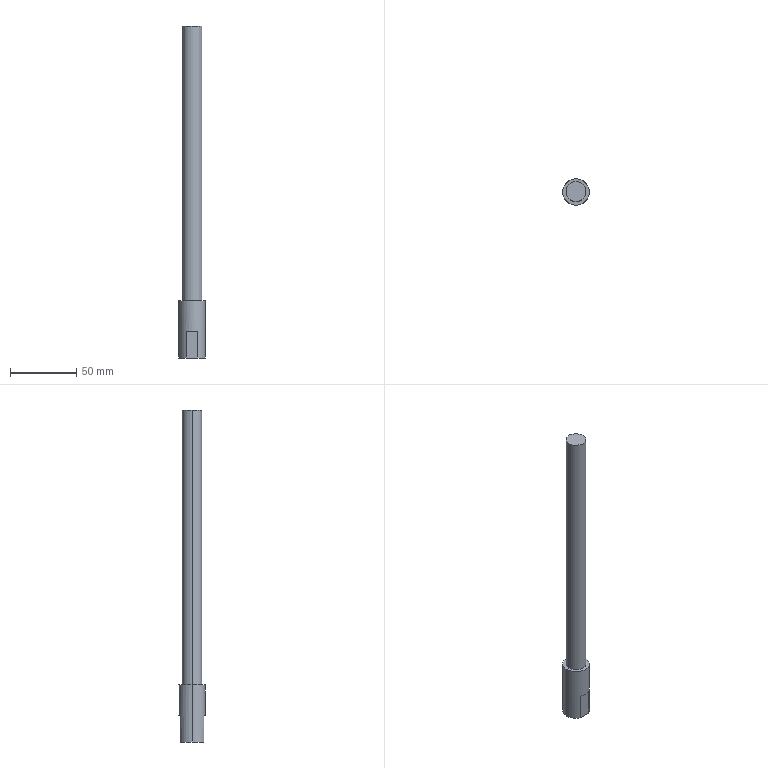Part | SolidWorks | features ICE 2, 3DProfileFeature 1, Extrusion 1, HoleWzd 1 | 1 solid | 17 faces | box 20 x 20 x 250 mm | volume 49162 mm3 | plane 7 | cylinder 6 | cone 4 | commonest cylinder face diameters 6.8 x2 15 x2 20 x2
STEP:
#1=CARTESIAN_POINT('',(3.4,0.,-42.375));
#2=VERTEX_POINT('',#1);
#3=CARTESIAN_POINT('',(-3.4,0.,-42.375));
#4=VERTEX_POINT('',#3);
#5=CARTESIAN_POINT('',(0.,0.,-42.375));
#6=DIRECTION('',(0.,0.,-1.));
#7=DIRECTION('',(-1.,0.,0.));
#8=AXIS2_PLACEMENT_3D('',#5,#6,#7);
#9=CIRCLE('',#8,3.4);
#10=EDGE_CURVE('',#2,#4,#9,.T.);
#11=ORIENTED_EDGE('',*,*,#10,.F.);
#12=CARTESIAN_POINT('',(4.025,0.,-43.));
#13=VERTEX_POINT('',#12);
#14=CARTESIAN_POINT('',(4.025,0.,-43.));
#15=DIRECTION('',(0.7071,0.,-0.7071));
#16=VECTOR('',#15,1000.);
#17=LINE('',#14,#16);
#18=EDGE_CURVE('',#2,#13,#17,.T.);
#19=ORIENTED_EDGE('',*,*,#18,.T.);
#20=CARTESIAN_POINT('',(-4.025,0.,-43.));
#21=VERTEX_POINT('',#20);
#22=CARTESIAN_POINT('',(0.,0.,-43.));
#23=DIRECTION('',(0.,0.,-1.));
#24=DIRECTION('',(-1.,0.,0.));
#25=AXIS2_PLACEMENT_3D('',#22,#23,#24);
#26=CIRCLE('',#25,4.025);
#27=EDGE_CURVE('',#13,#21,#26,.T.);
#28=ORIENTED_EDGE('',*,*,#27,.T.);
#29=CARTESIAN_POINT('',(-4.025,0.,-43.));
#30=DIRECTION('',(-0.7071,0.,-0.7071));
#31=VECTOR('',#30,1000.);
#32=LINE('',#29,#31);
#33=EDGE_CURVE('',#4,#21,#32,.T.);
#34=ORIENTED_EDGE('',*,*,#33,.F.);
#35=EDGE_LOOP('',(#11,#19,#28,#34));
#36=FACE_OUTER_BOUND('',#35,.T.);
#37=CARTESIAN_POINT('',(0.,0.,-43.));
#38=DIRECTION('',(0.,0.,-1.));
#39=DIRECTION('',(-1.,0.,0.));
#40=AXIS2_PLACEMENT_3D('',#37,#38,#39);
#41=CONICAL_SURFACE('',#40,4.025,0.7854);
#42=ADVANCED_FACE('',(#36),#41,.F.);
#43=CARTESIAN_POINT('',(3.4,0.,-24.75));
#44=VERTEX_POINT('',#43);
#45=CARTESIAN_POINT('',(-3.4,0.,-24.75));
#46=VERTEX_POINT('',#45);
#47=CARTESIAN_POINT('',(0.,0.,-24.75));
#48=DIRECTION('',(0.,0.,-1.));
#49=DIRECTION('',(-1.,0.,0.));
#50=AXIS2_PLACEMENT_3D('',#47,#48,#49);
#51=CIRCLE('',#50,3.4);
#52=EDGE_CURVE('',#44,#46,#51,.T.);
#53=ORIENTED_EDGE('',*,*,#52,.F.);
#54=CARTESIAN_POINT('',(3.4,0.,-43.));
#55=DIRECTION('',(0.,0.,-1.));
#56=VECTOR('',#55,1000.);
#57=LINE('',#54,#56);
#58=EDGE_CURVE('',#44,#2,#57,.T.);
#59=ORIENTED_EDGE('',*,*,#58,.T.);
#60=ORIENTED_EDGE('',*,*,#10,.T.);
#61=CARTESIAN_POINT('',(-3.4,0.,-43.));
#62=DIRECTION('',(0.,0.,-1.));
#63=VECTOR('',#62,1000.);
#64=LINE('',#61,#63);
#65=EDGE_CURVE('',#46,#4,#64,.T.);
#66=ORIENTED_EDGE('',*,*,#65,.F.);
#67=EDGE_LOOP('',(#53,#59,#60,#66));
#68=FACE_OUTER_BOUND('',#67,.T.);
#69=CARTESIAN_POINT('',(0.,0.,-43.));
#70=DIRECTION('',(0.,0.,-1.));
#71=DIRECTION('',(-1.,0.,0.));
#72=AXIS2_PLACEMENT_3D('',#69,#70,#71);
#73=CYLINDRICAL_SURFACE('',#72,3.4);
#74=ADVANCED_FACE('',(#68),#73,.F.);
#75=CARTESIAN_POINT('',(0.,0.,-22.707));
#76=VERTEX_POINT('',#75);
#77=CARTESIAN_POINT('',(-3.4,0.,-24.75));
#78=DIRECTION('',(-0.8572,0.,-0.515));
#79=VECTOR('',#78,1000.);
#80=LINE('',#77,#79);
#81=EDGE_CURVE('',#76,#46,#80,.T.);
#82=ORIENTED_EDGE('',*,*,#81,.F.);
#83=CARTESIAN_POINT('',(3.4,0.,-24.75));
#84=DIRECTION('',(0.8572,0.,-0.515));
#85=VECTOR('',#84,1000.);
#86=LINE('',#83,#85);
#87=EDGE_CURVE('',#76,#44,#86,.T.);
#88=ORIENTED_EDGE('',*,*,#87,.T.);
#89=ORIENTED_EDGE('',*,*,#52,.T.);
#90=EDGE_LOOP('',(#82,#88,#89));
#91=FACE_OUTER_BOUND('',#90,.T.);
#92=CARTESIAN_POINT('',(0.,0.,-24.75));
#93=DIRECTION('',(0.,0.,-1.));
#94=DIRECTION('',(-1.,0.,0.));
#95=AXIS2_PLACEMENT_3D('',#92,#93,#94);
#96=CONICAL_SURFACE('',#95,3.4,1.03);
#97=ADVANCED_FACE('',(#91),#96,.F.);
#98=CARTESIAN_POINT('',(7.5,0.,207.));
#99=VERTEX_POINT('',#98);
#100=CARTESIAN_POINT('',(-7.5,0.,207.));
#101=VERTEX_POINT('',#100);
#102=CARTESIAN_POINT('',(0.,0.,207.));
#103=DIRECTION('',(0.,0.,1.));
#104=DIRECTION('',(1.,0.,0.));
#105=AXIS2_PLACEMENT_3D('',#102,#103,#104);
#106=CIRCLE('',#105,7.5);
#107=EDGE_CURVE('',#99,#101,#106,.T.);
#108=ORIENTED_EDGE('',*,*,#107,.F.);
#109=CARTESIAN_POINT('',(7.5,0.,0.));
#110=VERTEX_POINT('',#109);
#111=CARTESIAN_POINT('',(7.5,0.,207.));
#112=DIRECTION('',(0.,0.,-1.));
#113=VECTOR('',#112,1000.);
#114=LINE('',#111,#113);
#115=EDGE_CURVE('',#99,#110,#114,.T.);
#116=ORIENTED_EDGE('',*,*,#115,.T.);
#117=CARTESIAN_POINT('',(-7.5,0.,0.));
#118=VERTEX_POINT('',#117);
#119=CARTESIAN_POINT('',(0.,0.,0.));
#120=DIRECTION('',(0.,0.,1.));
#121=DIRECTION('',(1.,0.,0.));
#122=AXIS2_PLACEMENT_3D('',#119,#120,#121);
#123=CIRCLE('',#122,7.5);
#124=EDGE_CURVE('',#110,#118,#123,.T.);
#125=ORIENTED_EDGE('',*,*,#124,.T.);
#126=CARTESIAN_POINT('',(-7.5,0.,207.));
#127=DIRECTION('',(0.,0.,-1.));
#128=VECTOR('',#127,1000.);
#129=LINE('',#126,#128);
#130=EDGE_CURVE('',#101,#118,#129,.T.);
#131=ORIENTED_EDGE('',*,*,#130,.F.);
#132=EDGE_LOOP('',(#108,#116,#125,#131));
#133=FACE_OUTER_BOUND('',#132,.T.);
#134=CARTESIAN_POINT('',(0.,0.,207.));
#135=DIRECTION('',(0.,0.,-1.));
#136=DIRECTION('',(-1.,0.,0.));
#137=AXIS2_PLACEMENT_3D('',#134,#135,#136);
#138=CYLINDRICAL_SURFACE('',#137,7.5);
#139=ADVANCED_FACE('',(#133),#138,.T.);
#140=CARTESIAN_POINT('',(-10.,0.,-43.));
#141=VERTEX_POINT('',#140);
#142=CARTESIAN_POINT('',(-4.359,9.,-43.));
#143=VERTEX_POINT('',#142);
#144=CARTESIAN_POINT('',(0.,0.,-43.));
#145=DIRECTION('',(0.,0.,-1.));
#146=DIRECTION('',(-1.,0.,0.));
#147=AXIS2_PLACEMENT_3D('',#144,#145,#146);
#148=CIRCLE('',#147,10.);
#149=EDGE_CURVE('',#141,#143,#148,.T.);
#150=ORIENTED_EDGE('',*,*,#149,.F.);
#151=CARTESIAN_POINT('',(-10.,0.,0.));
#152=VERTEX_POINT('',#151);
#153=CARTESIAN_POINT('',(-10.,0.,-43.));
#154=DIRECTION('',(0.,0.,1.));
#155=VECTOR('',#154,1000.);
#156=LINE('',#153,#155);
#157=EDGE_CURVE('',#141,#152,#156,.T.);
#158=ORIENTED_EDGE('',*,*,#157,.T.);
#159=CARTESIAN_POINT('',(10.,0.,0.));
#160=VERTEX_POINT('',#159);
#161=CARTESIAN_POINT('',(0.,0.,0.));
#162=DIRECTION('',(0.,0.,-1.));
#163=DIRECTION('',(-1.,0.,0.));
#164=AXIS2_PLACEMENT_3D('',#161,#162,#163);
#165=CIRCLE('',#164,10.);
#166=EDGE_CURVE('',#152,#160,#165,.T.);
#167=ORIENTED_EDGE('',*,*,#166,.T.);
#168=CARTESIAN_POINT('',(10.,0.,-43.));
#169=VERTEX_POINT('',#168);
#170=CARTESIAN_POINT('',(10.,0.,-43.));
#171=DIRECTION('',(0.,0.,1.));
#172=VECTOR('',#171,1000.);
#173=LINE('',#170,#172);
#174=EDGE_CURVE('',#169,#160,#173,.T.);
#175=ORIENTED_EDGE('',*,*,#174,.F.);
#176=CARTESIAN_POINT('',(4.359,9.,-43.));
#177=VERTEX_POINT('',#176);
#178=CARTESIAN_POINT('',(0.,0.,-43.));
#179=DIRECTION('',(0.,0.,-1.));
#180=DIRECTION('',(-1.,0.,0.));
#181=AXIS2_PLACEMENT_3D('',#178,#179,#180);
#182=CIRCLE('',#181,10.);
#183=EDGE_CURVE('',#177,#169,#182,.T.);
#184=ORIENTED_EDGE('',*,*,#183,.F.);
#185=CARTESIAN_POINT('',(4.359,9.,-23.));
#186=VERTEX_POINT('',#185);
#187=CARTESIAN_POINT('',(4.359,9.,-43.));
#188=DIRECTION('',(0.,0.,-1.));
#189=VECTOR('',#188,1000.);
#190=LINE('',#187,#189);
#191=EDGE_CURVE('',#186,#177,#190,.T.);
#192=ORIENTED_EDGE('',*,*,#191,.F.);
#193=CARTESIAN_POINT('',(-4.359,9.,-23.));
#194=VERTEX_POINT('',#193);
#195=CARTESIAN_POINT('',(0.,0.,-23.));
#196=DIRECTION('',(0.,0.,-1.));
#197=DIRECTION('',(-1.,0.,0.));
#198=AXIS2_PLACEMENT_3D('',#195,#196,#197);
#199=CIRCLE('',#198,10.);
#200=EDGE_CURVE('',#194,#186,#199,.T.);
#201=ORIENTED_EDGE('',*,*,#200,.F.);
#202=CARTESIAN_POINT('',(-4.359,9.,-43.));
#203=DIRECTION('',(0.,0.,1.));
#204=VECTOR('',#203,1000.);
#205=LINE('',#202,#204);
#206=EDGE_CURVE('',#143,#194,#205,.T.);
#207=ORIENTED_EDGE('',*,*,#206,.F.);
#208=EDGE_LOOP('',(#150,#158,#167,#175,#184,#192,#201,#207));
#209=FACE_OUTER_BOUND('',#208,.T.);
#210=CARTESIAN_POINT('',(0.,0.,-43.));
#211=DIRECTION('',(0.,0.,1.));
#212=DIRECTION('',(1.,0.,0.));
#213=AXIS2_PLACEMENT_3D('',#210,#211,#212);
#214=CYLINDRICAL_SURFACE('',#213,10.);
#215=ADVANCED_FACE('',(#209),#214,.T.);
#216=ORIENTED_EDGE('',*,*,#157,.F.);
#217=CARTESIAN_POINT('',(-4.359,-9.,-43.));
#218=VERTEX_POINT('',#217);
#219=CARTESIAN_POINT('',(0.,0.,-43.));
#220=DIRECTION('',(0.,0.,-1.));
#221=DIRECTION('',(-1.,0.,0.));
#222=AXIS2_PLACEMENT_3D('',#219,#220,#221);
#223=CIRCLE('',#222,10.);
#224=EDGE_CURVE('',#218,#141,#223,.T.);
#225=ORIENTED_EDGE('',*,*,#224,.F.);
#226=CARTESIAN_POINT('',(-4.359,-9.,-23.));
#227=VERTEX_POINT('',#226);
#228=CARTESIAN_POINT('',(-4.359,-9.,-43.));
#229=DIRECTION('',(0.,0.,-1.));
#230=VECTOR('',#229,1000.);
#231=LINE('',#228,#230);
#232=EDGE_CURVE('',#227,#218,#231,.T.);
#233=ORIENTED_EDGE('',*,*,#232,.F.);
#234=CARTESIAN_POINT('',(4.359,-9.,-23.));
#235=VERTEX_POINT('',#234);
#236=CARTESIAN_POINT('',(0.,0.,-23.));
#237=DIRECTION('',(0.,0.,-1.));
#238=DIRECTION('',(-1.,0.,0.));
#239=AXIS2_PLACEMENT_3D('',#236,#237,#238);
#240=CIRCLE('',#239,10.);
#241=EDGE_CURVE('',#235,#227,#240,.T.);
#242=ORIENTED_EDGE('',*,*,#241,.F.);
#243=CARTESIAN_POINT('',(4.359,-9.,-43.));
#244=VERTEX_POINT('',#243);
#245=CARTESIAN_POINT('',(4.359,-9.,-43.));
#246=DIRECTION('',(0.,0.,1.));
#247=VECTOR('',#246,1000.);
#248=LINE('',#245,#247);
#249=EDGE_CURVE('',#244,#235,#248,.T.);
#250=ORIENTED_EDGE('',*,*,#249,.F.);
#251=CARTESIAN_POINT('',(0.,0.,-43.));
#252=DIRECTION('',(0.,0.,-1.));
#253=DIRECTION('',(-1.,0.,0.));
#254=AXIS2_PLACEMENT_3D('',#251,#252,#253);
#255=CIRCLE('',#254,10.);
#256=EDGE_CURVE('',#169,#244,#255,.T.);
#257=ORIENTED_EDGE('',*,*,#256,.F.);
#258=ORIENTED_EDGE('',*,*,#174,.T.);
#259=CARTESIAN_POINT('',(0.,0.,0.));
#260=DIRECTION('',(0.,0.,-1.));
#261=DIRECTION('',(-1.,0.,0.));
#262=AXIS2_PLACEMENT_3D('',#259,#260,#261);
#263=CIRCLE('',#262,10.);
#264=EDGE_CURVE('',#160,#152,#263,.T.);
#265=ORIENTED_EDGE('',*,*,#264,.T.);
#266=EDGE_LOOP('',(#216,#225,#233,#242,#250,#257,#258,#265));
#267=FACE_OUTER_BOUND('',#266,.T.);
#268=CARTESIAN_POINT('',(0.,0.,-43.));
#269=DIRECTION('',(0.,0.,1.));
#270=DIRECTION('',(1.,0.,0.));
#271=AXIS2_PLACEMENT_3D('',#268,#269,#270);
#272=CYLINDRICAL_SURFACE('',#271,10.);
#273=ADVANCED_FACE('',(#267),#272,.T.);
#274=CARTESIAN_POINT('',(0.,0.,-43.));
#275=DIRECTION('',(0.,0.,-1.));
#276=DIRECTION('',(-1.,0.,0.));
#277=AXIS2_PLACEMENT_3D('',#274,#275,#276);
#278=CIRCLE('',#277,4.025);
#279=EDGE_CURVE('',#21,#13,#278,.T.);
#280=ORIENTED_EDGE('',*,*,#279,.F.);
#281=ORIENTED_EDGE('',*,*,#27,.F.);
#282=EDGE_LOOP('',(#280,#281));
#283=FACE_BOUND('',#282,.T.);
#284=ORIENTED_EDGE('',*,*,#183,.T.);
#285=ORIENTED_EDGE('',*,*,#256,.T.);
#286=CARTESIAN_POINT('',(0.,-9.,-43.));
#287=DIRECTION('',(-1.,0.,0.));
#288=VECTOR('',#287,1000.);
#289=LINE('',#286,#288);
#290=EDGE_CURVE('',#244,#218,#289,.T.);
#291=ORIENTED_EDGE('',*,*,#290,.T.);
#292=ORIENTED_EDGE('',*,*,#224,.T.);
#293=ORIENTED_EDGE('',*,*,#149,.T.);
#294=CARTESIAN_POINT('',(0.,9.,-43.));
#295=DIRECTION('',(1.,0.,0.));
#296=VECTOR('',#295,1000.);
#297=LINE('',#294,#296);
#298=EDGE_CURVE('',#143,#177,#297,.T.);
#299=ORIENTED_EDGE('',*,*,#298,.T.);
#300=EDGE_LOOP('',(#284,#285,#291,#292,#293,#299));
#301=FACE_OUTER_BOUND('',#300,.T.);
#302=CARTESIAN_POINT('',(0.,0.,-43.));
#303=DIRECTION('',(0.,0.,-1.));
#304=DIRECTION('',(-1.,0.,0.));
#305=AXIS2_PLACEMENT_3D('',#302,#303,#304);
#306=PLANE('',#305);
#307=ADVANCED_FACE('',(#283,#301),#306,.T.);
#308=ORIENTED_EDGE('',*,*,#115,.F.);
#309=CARTESIAN_POINT('',(0.,0.,207.));
#310=DIRECTION('',(0.,0.,1.));
#311=DIRECTION('',(1.,0.,0.));
#312=AXIS2_PLACEMENT_3D('',#309,#310,#311);
#313=CIRCLE('',#312,7.5);
#314=EDGE_CURVE('',#101,#99,#313,.T.);
#315=ORIENTED_EDGE('',*,*,#314,.F.);
#316=ORIENTED_EDGE('',*,*,#130,.T.);
#317=CARTESIAN_POINT('',(0.,0.,0.));
#318=DIRECTION('',(0.,0.,1.));
#319=DIRECTION('',(1.,0.,0.));
#320=AXIS2_PLACEMENT_3D('',#317,#318,#319);
#321=CIRCLE('',#320,7.5);
#322=EDGE_CURVE('',#118,#110,#321,.T.);
#323=ORIENTED_EDGE('',*,*,#322,.T.);
#324=EDGE_LOOP('',(#308,#315,#316,#323));
#325=FACE_OUTER_BOUND('',#324,.T.);
#326=CARTESIAN_POINT('',(0.,0.,207.));
#327=DIRECTION('',(0.,0.,-1.));
#328=DIRECTION('',(-1.,0.,0.));
#329=AXIS2_PLACEMENT_3D('',#326,#327,#328);
#330=CYLINDRICAL_SURFACE('',#329,7.5);
#331=ADVANCED_FACE('',(#325),#330,.T.);
#332=ORIENTED_EDGE('',*,*,#314,.T.);
#333=ORIENTED_EDGE('',*,*,#107,.T.);
#334=EDGE_LOOP('',(#332,#333));
#335=FACE_OUTER_BOUND('',#334,.T.);
#336=CARTESIAN_POINT('',(0.,0.,207.));
#337=DIRECTION('',(0.,0.,1.));
#338=DIRECTION('',(1.,0.,0.));
#339=AXIS2_PLACEMENT_3D('',#336,#337,#338);
#340=PLANE('',#339);
#341=ADVANCED_FACE('',(#335),#340,.T.);
#342=ORIENTED_EDGE('',*,*,#322,.F.);
#343=ORIENTED_EDGE('',*,*,#124,.F.);
#344=EDGE_LOOP('',(#342,#343));
#345=FACE_BOUND('',#344,.T.);
#346=ORIENTED_EDGE('',*,*,#264,.F.);
#347=ORIENTED_EDGE('',*,*,#166,.F.);
#348=EDGE_LOOP('',(#346,#347));
#349=FACE_OUTER_BOUND('',#348,.T.);
#350=CARTESIAN_POINT('',(0.,0.,0.));
#351=DIRECTION('',(0.,0.,-1.));
#352=DIRECTION('',(-1.,0.,0.));
#353=AXIS2_PLACEMENT_3D('',#350,#351,#352);
#354=PLANE('',#353);
#355=ADVANCED_FACE('',(#345,#349),#354,.F.);
#356=ORIENTED_EDGE('',*,*,#206,.T.);
#357=CARTESIAN_POINT('',(11.5,9.,-23.));
#358=DIRECTION('',(1.,0.,0.));
#359=VECTOR('',#358,1000.);
#360=LINE('',#357,#359);
#361=EDGE_CURVE('',#194,#186,#360,.T.);
#362=ORIENTED_EDGE('',*,*,#361,.T.);
#363=ORIENTED_EDGE('',*,*,#191,.T.);
#364=ORIENTED_EDGE('',*,*,#298,.F.);
#365=EDGE_LOOP('',(#356,#362,#363,#364));
#366=FACE_OUTER_BOUND('',#365,.T.);
#367=CARTESIAN_POINT('',(11.5,9.,-23.));
#368=DIRECTION('',(0.,1.,0.));
#369=DIRECTION('',(0.,0.,1.));
#370=AXIS2_PLACEMENT_3D('',#367,#368,#369);
#371=PLANE('',#370);
#372=ADVANCED_FACE('',(#366),#371,.T.);
#373=ORIENTED_EDGE('',*,*,#200,.T.);
#374=ORIENTED_EDGE('',*,*,#361,.F.);
#375=EDGE_LOOP('',(#373,#374));
#376=FACE_OUTER_BOUND('',#375,.T.);
#377=CARTESIAN_POINT('',(0.,0.,-23.));
#378=DIRECTION('',(0.,0.,-1.));
#379=DIRECTION('',(-1.,0.,0.));
#380=AXIS2_PLACEMENT_3D('',#377,#378,#379);
#381=PLANE('',#380);
#382=ADVANCED_FACE('',(#376),#381,.T.);
#383=ORIENTED_EDGE('',*,*,#241,.T.);
#384=CARTESIAN_POINT('',(11.5,-9.,-23.));
#385=DIRECTION('',(-1.,0.,0.));
#386=VECTOR('',#385,1000.);
#387=LINE('',#384,#386);
#388=EDGE_CURVE('',#235,#227,#387,.T.);
#389=ORIENTED_EDGE('',*,*,#388,.F.);
#390=EDGE_LOOP('',(#383,#389));
#391=FACE_OUTER_BOUND('',#390,.T.);
#392=CARTESIAN_POINT('',(0.,0.,-23.));
#393=DIRECTION('',(0.,0.,-1.));
#394=DIRECTION('',(-1.,0.,0.));
#395=AXIS2_PLACEMENT_3D('',#392,#393,#394);
#396=PLANE('',#395);
#397=ADVANCED_FACE('',(#391),#396,.T.);
#398=ORIENTED_EDGE('',*,*,#249,.T.);
#399=ORIENTED_EDGE('',*,*,#388,.T.);
#400=ORIENTED_EDGE('',*,*,#232,.T.);
#401=ORIENTED_EDGE('',*,*,#290,.F.);
#402=EDGE_LOOP('',(#398,#399,#400,#401));
#403=FACE_OUTER_BOUND('',#402,.T.);
#404=CARTESIAN_POINT('',(11.5,-9.,-23.));
#405=DIRECTION('',(0.,-1.,0.));
#406=DIRECTION('',(0.,0.,-1.));
#407=AXIS2_PLACEMENT_3D('',#404,#405,#406);
#408=PLANE('',#407);
#409=ADVANCED_FACE('',(#403),#408,.T.);
#410=ORIENTED_EDGE('',*,*,#87,.F.);
#411=ORIENTED_EDGE('',*,*,#81,.T.);
#412=CARTESIAN_POINT('',(0.,0.,-24.75));
#413=DIRECTION('',(0.,0.,-1.));
#414=DIRECTION('',(-1.,0.,0.));
#415=AXIS2_PLACEMENT_3D('',#412,#413,#414);
#416=CIRCLE('',#415,3.4);
#417=EDGE_CURVE('',#46,#44,#416,.T.);
#418=ORIENTED_EDGE('',*,*,#417,.T.);
#419=EDGE_LOOP('',(#410,#411,#418));
#420=FACE_OUTER_BOUND('',#419,.T.);
#421=CARTESIAN_POINT('',(0.,0.,-24.75));
#422=DIRECTION('',(0.,0.,-1.));
#423=DIRECTION('',(-1.,0.,0.));
#424=AXIS2_PLACEMENT_3D('',#421,#422,#423);
#425=CONICAL_SURFACE('',#424,3.4,1.03);
#426=ADVANCED_FACE('',(#420),#425,.F.);
#427=ORIENTED_EDGE('',*,*,#58,.F.);
#428=ORIENTED_EDGE('',*,*,#417,.F.);
#429=ORIENTED_EDGE('',*,*,#65,.T.);
#430=CARTESIAN_POINT('',(0.,0.,-42.375));
#431=DIRECTION('',(0.,0.,-1.));
#432=DIRECTION('',(-1.,0.,0.));
#433=AXIS2_PLACEMENT_3D('',#430,#431,#432);
#434=CIRCLE('',#433,3.4);
#435=EDGE_CURVE('',#4,#2,#434,.T.);
#436=ORIENTED_EDGE('',*,*,#435,.T.);
#437=EDGE_LOOP('',(#427,#428,#429,#436));
#438=FACE_OUTER_BOUND('',#437,.T.);
#439=CARTESIAN_POINT('',(0.,0.,-43.));
#440=DIRECTION('',(0.,0.,-1.));
#441=DIRECTION('',(-1.,0.,0.));
#442=AXIS2_PLACEMENT_3D('',#439,#440,#441);
#443=CYLINDRICAL_SURFACE('',#442,3.4);
#444=ADVANCED_FACE('',(#438),#443,.F.);
#445=ORIENTED_EDGE('',*,*,#18,.F.);
#446=ORIENTED_EDGE('',*,*,#435,.F.);
#447=ORIENTED_EDGE('',*,*,#33,.T.);
#448=ORIENTED_EDGE('',*,*,#279,.T.);
#449=EDGE_LOOP('',(#445,#446,#447,#448));
#450=FACE_OUTER_BOUND('',#449,.T.);
#451=CARTESIAN_POINT('',(0.,0.,-43.));
#452=DIRECTION('',(0.,0.,-1.));
#453=DIRECTION('',(-1.,0.,0.));
#454=AXIS2_PLACEMENT_3D('',#451,#452,#453);
#455=CONICAL_SURFACE('',#454,4.025,0.7854);
#456=ADVANCED_FACE('',(#450),#455,.F.);
#457=CLOSED_SHELL('',(#42,#74,#97,#139,#215,#273,#307,#331,#341,#355,#372,#382,#397,#409,#426,#444,#456));
#458=MANIFOLD_SOLID_BREP('',#457);
#459=CARTESIAN_POINT('',(0.,0.,0.));
#460=DIRECTION('',(0.,0.,1.));
#461=DIRECTION('',(1.,0.,0.));
#462=AXIS2_PLACEMENT_3D('',#459,#460,#461);
#463=(LENGTH_UNIT()NAMED_UNIT(*)SI_UNIT(.MILLI.,.METRE.));
#464=UNCERTAINTY_MEASURE_WITH_UNIT(LENGTH_MEASURE(0.00001),#463,'','');
#465=(NAMED_UNIT(*)PLANE_ANGLE_UNIT()SI_UNIT($,.RADIAN.));
#466=(NAMED_UNIT(*)SI_UNIT($,.STERADIAN.)SOLID_ANGLE_UNIT());
#467=(GEOMETRIC_REPRESENTATION_CONTEXT(3)GLOBAL_UNCERTAINTY_ASSIGNED_CONTEXT((#464))GLOBAL_UNIT_ASSIGNED_CONTEXT((#463,#465,#466))REPRESENTATION_CONTEXT('',''));
#468=ADVANCED_BREP_SHAPE_REPRESENTATION('',(#458,#462),#467);